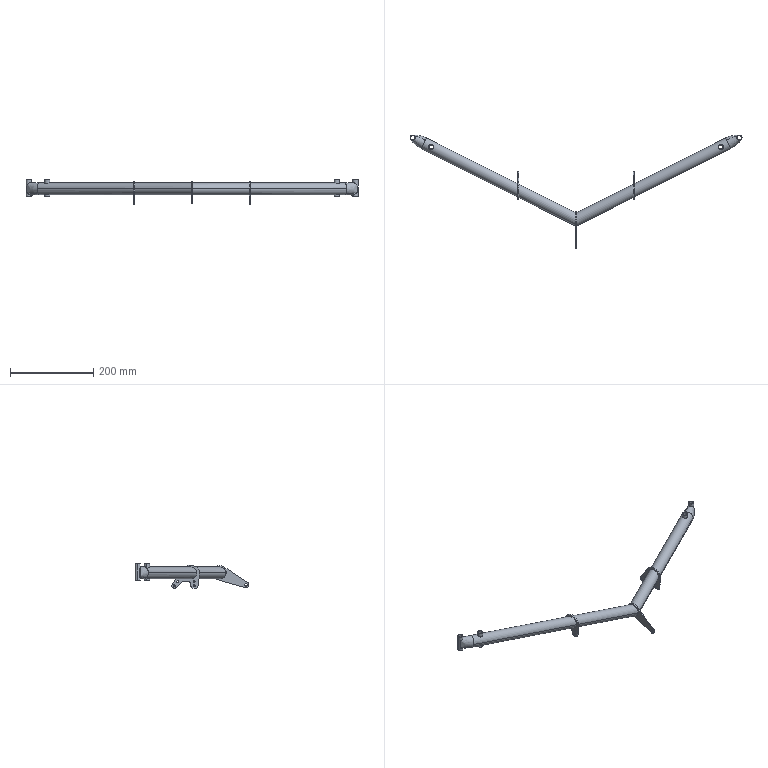Part | SolidWorks | features BaseBody 11 | 11 solids | 113 faces | box 799.556 x 274.686 x 59 mm | volume 147526 mm3 | cylinder 66 | plane 34 | spline 13 | commonest cylinder face diameters 12.7 x20 4.166 x16 10 x8 10.211 x8 25.629 x4 28.575 x4